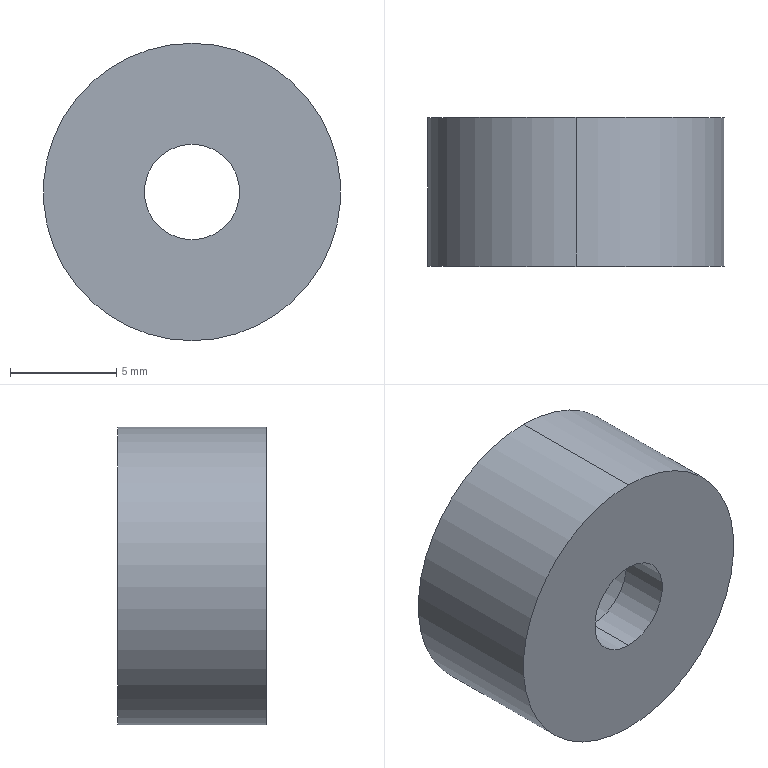Part | STEP file | 02-03 buffer pad block | 1 solid | 9 faces | box 14 x 7 x 14 mm | volume 808.175 mm3 | cylinder 6 | plane 3 | commonest cylinder face diameters 4.5 x2 8 x2 14 x2
STEP:
#1=CARTESIAN_POINT('',(0.,2.4,-4.));
#2=VERTEX_POINT('',#1);
#3=CARTESIAN_POINT('',(0.,2.4,4.));
#4=VERTEX_POINT('',#3);
#5=CARTESIAN_POINT('',(0.,2.4,0.));
#6=DIRECTION('',(0.,1.,0.));
#7=DIRECTION('',(0.,0.,1.));
#8=AXIS2_PLACEMENT_3D('',#5,#6,#7);
#9=CIRCLE('',#8,4.);
#10=EDGE_CURVE('',#2,#4,#9,.T.);
#11=ORIENTED_EDGE('',*,*,#10,.F.);
#12=CARTESIAN_POINT('',(0.,7.,-4.));
#13=VERTEX_POINT('',#12);
#14=CARTESIAN_POINT('',(0.,7.,-4.));
#15=DIRECTION('',(0.,1.,0.));
#16=VECTOR('',#15,1000.);
#17=LINE('',#14,#16);
#18=EDGE_CURVE('',#2,#13,#17,.T.);
#19=ORIENTED_EDGE('',*,*,#18,.T.);
#20=CARTESIAN_POINT('',(0.,7.,4.));
#21=VERTEX_POINT('',#20);
#22=CARTESIAN_POINT('',(0.,7.,0.));
#23=DIRECTION('',(0.,1.,0.));
#24=DIRECTION('',(0.,0.,1.));
#25=AXIS2_PLACEMENT_3D('',#22,#23,#24);
#26=CIRCLE('',#25,4.);
#27=EDGE_CURVE('',#13,#21,#26,.T.);
#28=ORIENTED_EDGE('',*,*,#27,.T.);
#29=CARTESIAN_POINT('',(0.,7.,4.));
#30=DIRECTION('',(0.,1.,0.));
#31=VECTOR('',#30,1000.);
#32=LINE('',#29,#31);
#33=EDGE_CURVE('',#4,#21,#32,.T.);
#34=ORIENTED_EDGE('',*,*,#33,.F.);
#35=EDGE_LOOP('',(#11,#19,#28,#34));
#36=FACE_OUTER_BOUND('',#35,.T.);
#37=CARTESIAN_POINT('',(0.,7.,0.));
#38=DIRECTION('',(0.,1.,0.));
#39=DIRECTION('',(0.,0.,1.));
#40=AXIS2_PLACEMENT_3D('',#37,#38,#39);
#41=CYLINDRICAL_SURFACE('',#40,4.);
#42=ADVANCED_FACE('',(#36),#41,.F.);
#43=CARTESIAN_POINT('',(0.,0.,-2.25));
#44=VERTEX_POINT('',#43);
#45=CARTESIAN_POINT('',(0.,0.,2.25));
#46=VERTEX_POINT('',#45);
#47=CARTESIAN_POINT('',(0.,0.,0.));
#48=DIRECTION('',(0.,1.,0.));
#49=DIRECTION('',(0.,0.,1.));
#50=AXIS2_PLACEMENT_3D('',#47,#48,#49);
#51=CIRCLE('',#50,2.25);
#52=EDGE_CURVE('',#44,#46,#51,.T.);
#53=ORIENTED_EDGE('',*,*,#52,.F.);
#54=CARTESIAN_POINT('',(0.,2.4,-2.25));
#55=VERTEX_POINT('',#54);
#56=CARTESIAN_POINT('',(0.,7.,-2.25));
#57=DIRECTION('',(0.,1.,0.));
#58=VECTOR('',#57,1000.);
#59=LINE('',#56,#58);
#60=EDGE_CURVE('',#44,#55,#59,.T.);
#61=ORIENTED_EDGE('',*,*,#60,.T.);
#62=CARTESIAN_POINT('',(0.,2.4,2.25));
#63=VERTEX_POINT('',#62);
#64=CARTESIAN_POINT('',(0.,2.4,0.));
#65=DIRECTION('',(0.,1.,0.));
#66=DIRECTION('',(0.,0.,1.));
#67=AXIS2_PLACEMENT_3D('',#64,#65,#66);
#68=CIRCLE('',#67,2.25);
#69=EDGE_CURVE('',#55,#63,#68,.T.);
#70=ORIENTED_EDGE('',*,*,#69,.T.);
#71=CARTESIAN_POINT('',(0.,7.,2.25));
#72=DIRECTION('',(0.,1.,0.));
#73=VECTOR('',#72,1000.);
#74=LINE('',#71,#73);
#75=EDGE_CURVE('',#46,#63,#74,.T.);
#76=ORIENTED_EDGE('',*,*,#75,.F.);
#77=EDGE_LOOP('',(#53,#61,#70,#76));
#78=FACE_OUTER_BOUND('',#77,.T.);
#79=CARTESIAN_POINT('',(0.,7.,0.));
#80=DIRECTION('',(0.,1.,0.));
#81=DIRECTION('',(0.,0.,1.));
#82=AXIS2_PLACEMENT_3D('',#79,#80,#81);
#83=CYLINDRICAL_SURFACE('',#82,2.25);
#84=ADVANCED_FACE('',(#78),#83,.F.);
#85=CARTESIAN_POINT('',(0.,7.,-7.));
#86=VERTEX_POINT('',#85);
#87=CARTESIAN_POINT('',(0.,7.,7.));
#88=VERTEX_POINT('',#87);
#89=CARTESIAN_POINT('',(0.,7.,0.));
#90=DIRECTION('',(0.,-1.,0.));
#91=DIRECTION('',(0.,0.,-1.));
#92=AXIS2_PLACEMENT_3D('',#89,#90,#91);
#93=CIRCLE('',#92,7.);
#94=EDGE_CURVE('',#86,#88,#93,.T.);
#95=ORIENTED_EDGE('',*,*,#94,.T.);
#96=CARTESIAN_POINT('',(0.,0.,7.));
#97=VERTEX_POINT('',#96);
#98=CARTESIAN_POINT('',(0.,0.,7.));
#99=DIRECTION('',(0.,-1.,0.));
#100=VECTOR('',#99,1000.);
#101=LINE('',#98,#100);
#102=EDGE_CURVE('',#88,#97,#101,.T.);
#103=ORIENTED_EDGE('',*,*,#102,.T.);
#104=CARTESIAN_POINT('',(0.,0.,-7.));
#105=VERTEX_POINT('',#104);
#106=CARTESIAN_POINT('',(0.,0.,0.));
#107=DIRECTION('',(0.,-1.,0.));
#108=DIRECTION('',(0.,0.,-1.));
#109=AXIS2_PLACEMENT_3D('',#106,#107,#108);
#110=CIRCLE('',#109,7.);
#111=EDGE_CURVE('',#105,#97,#110,.T.);
#112=ORIENTED_EDGE('',*,*,#111,.F.);
#113=CARTESIAN_POINT('',(0.,0.,-7.));
#114=DIRECTION('',(0.,-1.,0.));
#115=VECTOR('',#114,1000.);
#116=LINE('',#113,#115);
#117=EDGE_CURVE('',#86,#105,#116,.T.);
#118=ORIENTED_EDGE('',*,*,#117,.F.);
#119=EDGE_LOOP('',(#95,#103,#112,#118));
#120=FACE_OUTER_BOUND('',#119,.T.);
#121=CARTESIAN_POINT('',(0.,0.,0.));
#122=DIRECTION('',(0.,-1.,0.));
#123=DIRECTION('',(0.,0.,-1.));
#124=AXIS2_PLACEMENT_3D('',#121,#122,#123);
#125=CYLINDRICAL_SURFACE('',#124,7.);
#126=ADVANCED_FACE('',(#120),#125,.T.);
#127=CARTESIAN_POINT('',(0.,7.,0.));
#128=DIRECTION('',(0.,1.,0.));
#129=DIRECTION('',(0.,0.,1.));
#130=AXIS2_PLACEMENT_3D('',#127,#128,#129);
#131=CIRCLE('',#130,4.);
#132=EDGE_CURVE('',#21,#13,#131,.T.);
#133=ORIENTED_EDGE('',*,*,#132,.F.);
#134=ORIENTED_EDGE('',*,*,#27,.F.);
#135=EDGE_LOOP('',(#133,#134));
#136=FACE_BOUND('',#135,.T.);
#137=ORIENTED_EDGE('',*,*,#94,.F.);
#138=CARTESIAN_POINT('',(0.,7.,0.));
#139=DIRECTION('',(0.,-1.,0.));
#140=DIRECTION('',(0.,0.,-1.));
#141=AXIS2_PLACEMENT_3D('',#138,#139,#140);
#142=CIRCLE('',#141,7.);
#143=EDGE_CURVE('',#88,#86,#142,.T.);
#144=ORIENTED_EDGE('',*,*,#143,.F.);
#145=EDGE_LOOP('',(#137,#144));
#146=FACE_OUTER_BOUND('',#145,.T.);
#147=CARTESIAN_POINT('',(0.,7.,0.));
#148=DIRECTION('',(0.,1.,0.));
#149=DIRECTION('',(0.,0.,1.));
#150=AXIS2_PLACEMENT_3D('',#147,#148,#149);
#151=PLANE('',#150);
#152=ADVANCED_FACE('',(#136,#146),#151,.T.);
#153=ORIENTED_EDGE('',*,*,#102,.F.);
#154=ORIENTED_EDGE('',*,*,#143,.T.);
#155=ORIENTED_EDGE('',*,*,#117,.T.);
#156=CARTESIAN_POINT('',(0.,0.,0.));
#157=DIRECTION('',(0.,-1.,0.));
#158=DIRECTION('',(0.,0.,-1.));
#159=AXIS2_PLACEMENT_3D('',#156,#157,#158);
#160=CIRCLE('',#159,7.);
#161=EDGE_CURVE('',#97,#105,#160,.T.);
#162=ORIENTED_EDGE('',*,*,#161,.F.);
#163=EDGE_LOOP('',(#153,#154,#155,#162));
#164=FACE_OUTER_BOUND('',#163,.T.);
#165=CARTESIAN_POINT('',(0.,0.,0.));
#166=DIRECTION('',(0.,-1.,0.));
#167=DIRECTION('',(0.,0.,-1.));
#168=AXIS2_PLACEMENT_3D('',#165,#166,#167);
#169=CYLINDRICAL_SURFACE('',#168,7.);
#170=ADVANCED_FACE('',(#164),#169,.T.);
#171=CARTESIAN_POINT('',(0.,0.,0.));
#172=DIRECTION('',(0.,1.,0.));
#173=DIRECTION('',(0.,0.,1.));
#174=AXIS2_PLACEMENT_3D('',#171,#172,#173);
#175=CIRCLE('',#174,2.25);
#176=EDGE_CURVE('',#46,#44,#175,.T.);
#177=ORIENTED_EDGE('',*,*,#176,.T.);
#178=ORIENTED_EDGE('',*,*,#52,.T.);
#179=EDGE_LOOP('',(#177,#178));
#180=FACE_BOUND('',#179,.T.);
#181=ORIENTED_EDGE('',*,*,#111,.T.);
#182=ORIENTED_EDGE('',*,*,#161,.T.);
#183=EDGE_LOOP('',(#181,#182));
#184=FACE_OUTER_BOUND('',#183,.T.);
#185=CARTESIAN_POINT('',(7.,0.,0.));
#186=DIRECTION('',(0.,-1.,0.));
#187=DIRECTION('',(0.,0.,-1.));
#188=AXIS2_PLACEMENT_3D('',#185,#186,#187);
#189=PLANE('',#188);
#190=ADVANCED_FACE('',(#180,#184),#189,.T.);
#191=ORIENTED_EDGE('',*,*,#60,.F.);
#192=ORIENTED_EDGE('',*,*,#176,.F.);
#193=ORIENTED_EDGE('',*,*,#75,.T.);
#194=CARTESIAN_POINT('',(0.,2.4,0.));
#195=DIRECTION('',(0.,1.,0.));
#196=DIRECTION('',(0.,0.,1.));
#197=AXIS2_PLACEMENT_3D('',#194,#195,#196);
#198=CIRCLE('',#197,2.25);
#199=EDGE_CURVE('',#63,#55,#198,.T.);
#200=ORIENTED_EDGE('',*,*,#199,.T.);
#201=EDGE_LOOP('',(#191,#192,#193,#200));
#202=FACE_OUTER_BOUND('',#201,.T.);
#203=CARTESIAN_POINT('',(0.,7.,0.));
#204=DIRECTION('',(0.,1.,0.));
#205=DIRECTION('',(0.,0.,1.));
#206=AXIS2_PLACEMENT_3D('',#203,#204,#205);
#207=CYLINDRICAL_SURFACE('',#206,2.25);
#208=ADVANCED_FACE('',(#202),#207,.F.);
#209=ORIENTED_EDGE('',*,*,#199,.F.);
#210=ORIENTED_EDGE('',*,*,#69,.F.);
#211=EDGE_LOOP('',(#209,#210));
#212=FACE_BOUND('',#211,.T.);
#213=CARTESIAN_POINT('',(0.,2.4,0.));
#214=DIRECTION('',(0.,1.,0.));
#215=DIRECTION('',(0.,0.,1.));
#216=AXIS2_PLACEMENT_3D('',#213,#214,#215);
#217=CIRCLE('',#216,4.);
#218=EDGE_CURVE('',#4,#2,#217,.T.);
#219=ORIENTED_EDGE('',*,*,#218,.T.);
#220=ORIENTED_EDGE('',*,*,#10,.T.);
#221=EDGE_LOOP('',(#219,#220));
#222=FACE_OUTER_BOUND('',#221,.T.);
#223=CARTESIAN_POINT('',(2.25,2.4,0.));
#224=DIRECTION('',(0.,-1.,0.));
#225=DIRECTION('',(0.,0.,-1.));
#226=AXIS2_PLACEMENT_3D('',#223,#224,#225);
#227=PLANE('',#226);
#228=ADVANCED_FACE('',(#212,#222),#227,.F.);
#229=ORIENTED_EDGE('',*,*,#18,.F.);
#230=ORIENTED_EDGE('',*,*,#218,.F.);
#231=ORIENTED_EDGE('',*,*,#33,.T.);
#232=ORIENTED_EDGE('',*,*,#132,.T.);
#233=EDGE_LOOP('',(#229,#230,#231,#232));
#234=FACE_OUTER_BOUND('',#233,.T.);
#235=CARTESIAN_POINT('',(0.,7.,0.));
#236=DIRECTION('',(0.,1.,0.));
#237=DIRECTION('',(0.,0.,1.));
#238=AXIS2_PLACEMENT_3D('',#235,#236,#237);
#239=CYLINDRICAL_SURFACE('',#238,4.);
#240=ADVANCED_FACE('',(#234),#239,.F.);
#241=CLOSED_SHELL('',(#42,#84,#126,#152,#170,#190,#208,#228,#240));
#242=MANIFOLD_SOLID_BREP('',#241);
#243=CARTESIAN_POINT('',(0.,0.,0.));
#244=DIRECTION('',(0.,0.,1.));
#245=DIRECTION('',(1.,0.,0.));
#246=AXIS2_PLACEMENT_3D('',#243,#244,#245);
#247=(LENGTH_UNIT()NAMED_UNIT(*)SI_UNIT(.MILLI.,.METRE.));
#248=UNCERTAINTY_MEASURE_WITH_UNIT(LENGTH_MEASURE(0.00001),#247,'','');
#249=(NAMED_UNIT(*)PLANE_ANGLE_UNIT()SI_UNIT($,.RADIAN.));
#250=(NAMED_UNIT(*)SI_UNIT($,.STERADIAN.)SOLID_ANGLE_UNIT());
#251=(GEOMETRIC_REPRESENTATION_CONTEXT(3)GLOBAL_UNCERTAINTY_ASSIGNED_CONTEXT((#248))GLOBAL_UNIT_ASSIGNED_CONTEXT((#247,#249,#250))REPRESENTATION_CONTEXT('',''));
#252=ADVANCED_BREP_SHAPE_REPRESENTATION('',(#242,#246),#251);